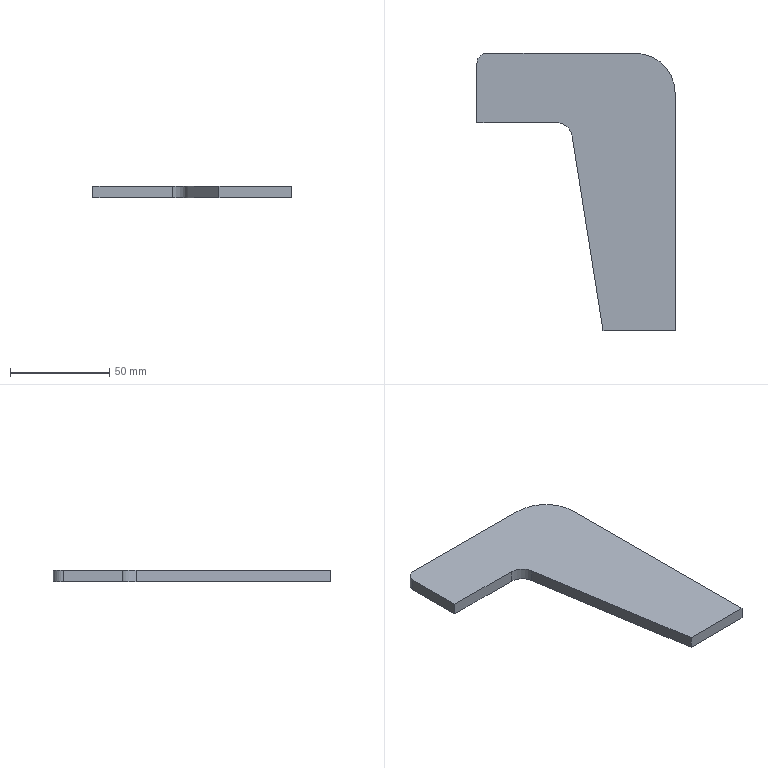Part | STEP file | 02-Reinforcing rib 1 | 1 solid | 11 faces | box 100 x 140 x 6 mm | volume 48661 mm3 | plane 8 | cylinder 3 | commonest cylinder face diameters 10 x1 16 x1 40 x1
STEP:
#1=CARTESIAN_POINT('',(0.,0.,0.));
#2=DIRECTION('',(0.,0.,1.));
#3=DIRECTION('',(1.,0.,0.));
#4=AXIS2_PLACEMENT_3D('',#1,#2,#3);
#5=CARTESIAN_POINT('',(0.,0.,0.));
#6=VERTEX_POINT('',#5);
#7=CARTESIAN_POINT('',(40.167,0.,0.));
#8=VERTEX_POINT('',#7);
#9=CARTESIAN_POINT('',(47.,0.,0.));
#10=DIRECTION('',(1.,0.,0.));
#11=VECTOR('',#10,1.);
#12=LINE('',#9,#11);
#13=CARTESIAN_POINT('',(47.,0.,6.));
#14=DIRECTION('',(0.,1.,0.));
#15=DIRECTION('',(-1.,0.,0.));
#16=AXIS2_PLACEMENT_3D('',#13,#14,#15);
#17=PLANE('',#16);
#18=CARTESIAN_POINT('',(0.,-6.));
#19=DIRECTION('',(-1.,0.));
#20=VECTOR('',#19,1.);
#21=LINE('',#18,#20);
#22=(GEOMETRIC_REPRESENTATION_CONTEXT(2)PARAMETRIC_REPRESENTATION_CONTEXT()REPRESENTATION_CONTEXT('',''));
#23=DEFINITIONAL_REPRESENTATION('',(#21),#22);
#24=PCURVE('',#17,#23);
#25=CARTESIAN_POINT('',(0.,0.,0.));
#26=DIRECTION('',(0.,0.,-1.));
#27=DIRECTION('',(-1.,0.,0.));
#28=AXIS2_PLACEMENT_3D('',#25,#26,#27);
#29=PLANE('',#28);
#30=CARTESIAN_POINT('',(-47.,0.));
#31=DIRECTION('',(-1.,0.));
#32=VECTOR('',#31,1.);
#33=LINE('',#30,#32);
#34=(GEOMETRIC_REPRESENTATION_CONTEXT(2)PARAMETRIC_REPRESENTATION_CONTEXT()REPRESENTATION_CONTEXT('',''));
#35=DEFINITIONAL_REPRESENTATION('',(#33),#34);
#36=PCURVE('',#29,#35);
#37=SURFACE_CURVE('',#12,(#24,#36),.PCURVE_S1.);
#38=EDGE_CURVE('',#6,#8,#37,.T.);
#39=ORIENTED_EDGE('',*,*,#38,.T.);
#40=CARTESIAN_POINT('',(40.167,0.,6.));
#41=VERTEX_POINT('',#40);
#42=CARTESIAN_POINT('',(40.167,0.,6.));
#43=DIRECTION('',(0.,0.,1.));
#44=VECTOR('',#43,1.);
#45=LINE('',#42,#44);
#46=CARTESIAN_POINT('',(6.833,0.));
#47=DIRECTION('',(0.,1.));
#48=VECTOR('',#47,1.);
#49=LINE('',#46,#48);
#50=(GEOMETRIC_REPRESENTATION_CONTEXT(2)PARAMETRIC_REPRESENTATION_CONTEXT()REPRESENTATION_CONTEXT('',''));
#51=DEFINITIONAL_REPRESENTATION('',(#49),#50);
#52=PCURVE('',#17,#51);
#53=CARTESIAN_POINT('',(40.167,-8.,6.));
#54=DIRECTION('',(0.,0.,1.));
#55=DIRECTION('',(1.,0.,0.));
#56=AXIS2_PLACEMENT_3D('',#53,#54,#55);
#57=CYLINDRICAL_SURFACE('',#56,8.);
#58=CARTESIAN_POINT('',(1.571,0.));
#59=DIRECTION('',(0.,1.));
#60=VECTOR('',#59,1.);
#61=LINE('',#58,#60);
#62=(GEOMETRIC_REPRESENTATION_CONTEXT(2)PARAMETRIC_REPRESENTATION_CONTEXT()REPRESENTATION_CONTEXT('',''));
#63=DEFINITIONAL_REPRESENTATION('',(#61),#62);
#64=PCURVE('',#57,#63);
#65=SURFACE_CURVE('',#45,(#52,#64),.PCURVE_S1.);
#66=EDGE_CURVE('',#8,#41,#65,.T.);
#67=ORIENTED_EDGE('',*,*,#66,.T.);
#68=CARTESIAN_POINT('',(0.,0.,6.));
#69=VERTEX_POINT('',#68);
#70=CARTESIAN_POINT('',(47.,0.,6.));
#71=DIRECTION('',(1.,0.,0.));
#72=VECTOR('',#71,1.);
#73=LINE('',#70,#72);
#74=CARTESIAN_POINT('',(0.,0.));
#75=DIRECTION('',(-1.,0.));
#76=VECTOR('',#75,1.);
#77=LINE('',#74,#76);
#78=(GEOMETRIC_REPRESENTATION_CONTEXT(2)PARAMETRIC_REPRESENTATION_CONTEXT()REPRESENTATION_CONTEXT('',''));
#79=DEFINITIONAL_REPRESENTATION('',(#77),#78);
#80=PCURVE('',#17,#79);
#81=CARTESIAN_POINT('',(0.,0.,6.));
#82=DIRECTION('',(0.,0.,-1.));
#83=DIRECTION('',(-1.,0.,0.));
#84=AXIS2_PLACEMENT_3D('',#81,#82,#83);
#85=PLANE('',#84);
#86=CARTESIAN_POINT('',(-47.,0.));
#87=DIRECTION('',(-1.,0.));
#88=VECTOR('',#87,1.);
#89=LINE('',#86,#88);
#90=(GEOMETRIC_REPRESENTATION_CONTEXT(2)PARAMETRIC_REPRESENTATION_CONTEXT()REPRESENTATION_CONTEXT('',''));
#91=DEFINITIONAL_REPRESENTATION('',(#89),#90);
#92=PCURVE('',#85,#91);
#93=SURFACE_CURVE('',#73,(#80,#92),.PCURVE_S1.);
#94=EDGE_CURVE('',#69,#41,#93,.T.);
#95=ORIENTED_EDGE('',*,*,#94,.F.);
#96=CARTESIAN_POINT('',(0.,0.,6.));
#97=DIRECTION('',(0.,0.,-1.));
#98=VECTOR('',#97,1.);
#99=LINE('',#96,#98);
#100=CARTESIAN_POINT('',(47.,0.));
#101=DIRECTION('',(0.,-1.));
#102=VECTOR('',#101,1.);
#103=LINE('',#100,#102);
#104=(GEOMETRIC_REPRESENTATION_CONTEXT(2)PARAMETRIC_REPRESENTATION_CONTEXT()REPRESENTATION_CONTEXT('',''));
#105=DEFINITIONAL_REPRESENTATION('',(#103),#104);
#106=PCURVE('',#17,#105);
#107=CARTESIAN_POINT('',(0.,0.,6.));
#108=DIRECTION('',(1.,0.,0.));
#109=DIRECTION('',(0.,0.,-1.));
#110=AXIS2_PLACEMENT_3D('',#107,#108,#109);
#111=PLANE('',#110);
#112=CARTESIAN_POINT('',(0.,0.));
#113=DIRECTION('',(1.,0.));
#114=VECTOR('',#113,1.);
#115=LINE('',#112,#114);
#116=(GEOMETRIC_REPRESENTATION_CONTEXT(2)PARAMETRIC_REPRESENTATION_CONTEXT()REPRESENTATION_CONTEXT('',''));
#117=DEFINITIONAL_REPRESENTATION('',(#115),#116);
#118=PCURVE('',#111,#117);
#119=SURFACE_CURVE('',#99,(#106,#118),.PCURVE_S1.);
#120=EDGE_CURVE('',#69,#6,#119,.T.);
#121=ORIENTED_EDGE('',*,*,#120,.T.);
#122=EDGE_LOOP('',(#39,#67,#95,#121));
#123=FACE_BOUND('',#122,.T.);
#124=ADVANCED_FACE('',(#123),#17,.F.);
#125=CARTESIAN_POINT('',(48.069,-6.749,6.));
#126=VERTEX_POINT('',#125);
#127=CARTESIAN_POINT('',(63.63,-105.,6.));
#128=VERTEX_POINT('',#127);
#129=CARTESIAN_POINT('',(63.63,-105.,6.));
#130=DIRECTION('',(0.1564,-0.9877,0.));
#131=VECTOR('',#130,1.);
#132=LINE('',#129,#131);
#133=CARTESIAN_POINT('',(63.63,-105.,6.));
#134=DIRECTION('',(0.9877,0.1564,0.));
#135=DIRECTION('',(-0.1564,0.9877,0.));
#136=AXIS2_PLACEMENT_3D('',#133,#134,#135);
#137=PLANE('',#136);
#138=CARTESIAN_POINT('',(0.,0.));
#139=DIRECTION('',(-1.,0.));
#140=VECTOR('',#139,1.);
#141=LINE('',#138,#140);
#142=(GEOMETRIC_REPRESENTATION_CONTEXT(2)PARAMETRIC_REPRESENTATION_CONTEXT()REPRESENTATION_CONTEXT('',''));
#143=DEFINITIONAL_REPRESENTATION('',(#141),#142);
#144=PCURVE('',#137,#143);
#145=CARTESIAN_POINT('',(-63.63,-105.));
#146=DIRECTION('',(-0.1564,-0.9877));
#147=VECTOR('',#146,1.);
#148=LINE('',#145,#147);
#149=(GEOMETRIC_REPRESENTATION_CONTEXT(2)PARAMETRIC_REPRESENTATION_CONTEXT()REPRESENTATION_CONTEXT('',''));
#150=DEFINITIONAL_REPRESENTATION('',(#148),#149);
#151=PCURVE('',#85,#150);
#152=SURFACE_CURVE('',#132,(#144,#151),.PCURVE_S1.);
#153=EDGE_CURVE('',#126,#128,#152,.T.);
#154=ORIENTED_EDGE('',*,*,#153,.F.);
#155=CARTESIAN_POINT('',(48.069,-6.749,0.));
#156=VERTEX_POINT('',#155);
#157=CARTESIAN_POINT('',(48.069,-6.749,0.));
#158=DIRECTION('',(0.,0.,-1.));
#159=VECTOR('',#158,1.);
#160=LINE('',#157,#159);
#161=CARTESIAN_POINT('',(99.476,-6.));
#162=DIRECTION('',(0.,-1.));
#163=VECTOR('',#162,1.);
#164=LINE('',#161,#163);
#165=(GEOMETRIC_REPRESENTATION_CONTEXT(2)PARAMETRIC_REPRESENTATION_CONTEXT()REPRESENTATION_CONTEXT('',''));
#166=DEFINITIONAL_REPRESENTATION('',(#164),#165);
#167=PCURVE('',#137,#166);
#168=CARTESIAN_POINT('',(0.1571,-6.));
#169=DIRECTION('',(0.,-1.));
#170=VECTOR('',#169,1.);
#171=LINE('',#168,#170);
#172=(GEOMETRIC_REPRESENTATION_CONTEXT(2)PARAMETRIC_REPRESENTATION_CONTEXT()REPRESENTATION_CONTEXT('',''));
#173=DEFINITIONAL_REPRESENTATION('',(#171),#172);
#174=PCURVE('',#57,#173);
#175=SURFACE_CURVE('',#160,(#167,#174),.PCURVE_S1.);
#176=EDGE_CURVE('',#126,#156,#175,.T.);
#177=ORIENTED_EDGE('',*,*,#176,.T.);
#178=CARTESIAN_POINT('',(63.63,-105.,0.));
#179=VERTEX_POINT('',#178);
#180=CARTESIAN_POINT('',(63.63,-105.,0.));
#181=DIRECTION('',(0.1564,-0.9877,0.));
#182=VECTOR('',#181,1.);
#183=LINE('',#180,#182);
#184=CARTESIAN_POINT('',(0.,-6.));
#185=DIRECTION('',(-1.,0.));
#186=VECTOR('',#185,1.);
#187=LINE('',#184,#186);
#188=(GEOMETRIC_REPRESENTATION_CONTEXT(2)PARAMETRIC_REPRESENTATION_CONTEXT()REPRESENTATION_CONTEXT('',''));
#189=DEFINITIONAL_REPRESENTATION('',(#187),#188);
#190=PCURVE('',#137,#189);
#191=CARTESIAN_POINT('',(-63.63,-105.));
#192=DIRECTION('',(-0.1564,-0.9877));
#193=VECTOR('',#192,1.);
#194=LINE('',#191,#193);
#195=(GEOMETRIC_REPRESENTATION_CONTEXT(2)PARAMETRIC_REPRESENTATION_CONTEXT()REPRESENTATION_CONTEXT('',''));
#196=DEFINITIONAL_REPRESENTATION('',(#194),#195);
#197=PCURVE('',#29,#196);
#198=SURFACE_CURVE('',#183,(#190,#197),.PCURVE_S1.);
#199=EDGE_CURVE('',#156,#179,#198,.T.);
#200=ORIENTED_EDGE('',*,*,#199,.T.);
#201=CARTESIAN_POINT('',(63.63,-105.,6.));
#202=DIRECTION('',(0.,0.,-1.));
#203=VECTOR('',#202,1.);
#204=LINE('',#201,#203);
#205=CARTESIAN_POINT('',(0.,0.));
#206=DIRECTION('',(0.,-1.));
#207=VECTOR('',#206,1.);
#208=LINE('',#205,#207);
#209=(GEOMETRIC_REPRESENTATION_CONTEXT(2)PARAMETRIC_REPRESENTATION_CONTEXT()REPRESENTATION_CONTEXT('',''));
#210=DEFINITIONAL_REPRESENTATION('',(#208),#209);
#211=PCURVE('',#137,#210);
#212=CARTESIAN_POINT('',(100.,-105.,6.));
#213=DIRECTION('',(0.,1.,0.));
#214=DIRECTION('',(0.,0.,1.));
#215=AXIS2_PLACEMENT_3D('',#212,#213,#214);
#216=PLANE('',#215);
#217=CARTESIAN_POINT('',(0.,-36.37));
#218=DIRECTION('',(-1.,0.));
#219=VECTOR('',#218,1.);
#220=LINE('',#217,#219);
#221=(GEOMETRIC_REPRESENTATION_CONTEXT(2)PARAMETRIC_REPRESENTATION_CONTEXT()REPRESENTATION_CONTEXT('',''));
#222=DEFINITIONAL_REPRESENTATION('',(#220),#221);
#223=PCURVE('',#216,#222);
#224=SURFACE_CURVE('',#204,(#211,#223),.PCURVE_S1.);
#225=EDGE_CURVE('',#128,#179,#224,.T.);
#226=ORIENTED_EDGE('',*,*,#225,.F.);
#227=EDGE_LOOP('',(#154,#177,#200,#226));
#228=FACE_BOUND('',#227,.T.);
#229=ADVANCED_FACE('',(#228),#137,.F.);
#230=CARTESIAN_POINT('',(100.,-105.,0.));
#231=VERTEX_POINT('',#230);
#232=CARTESIAN_POINT('',(100.,-105.,0.));
#233=DIRECTION('',(1.,0.,0.));
#234=VECTOR('',#233,1.);
#235=LINE('',#232,#234);
#236=CARTESIAN_POINT('',(-6.,0.));
#237=DIRECTION('',(0.,1.));
#238=VECTOR('',#237,1.);
#239=LINE('',#236,#238);
#240=(GEOMETRIC_REPRESENTATION_CONTEXT(2)PARAMETRIC_REPRESENTATION_CONTEXT()REPRESENTATION_CONTEXT('',''));
#241=DEFINITIONAL_REPRESENTATION('',(#239),#240);
#242=PCURVE('',#216,#241);
#243=CARTESIAN_POINT('',(-100.,-105.));
#244=DIRECTION('',(-1.,0.));
#245=VECTOR('',#244,1.);
#246=LINE('',#243,#245);
#247=(GEOMETRIC_REPRESENTATION_CONTEXT(2)PARAMETRIC_REPRESENTATION_CONTEXT()REPRESENTATION_CONTEXT('',''));
#248=DEFINITIONAL_REPRESENTATION('',(#246),#247);
#249=PCURVE('',#29,#248);
#250=SURFACE_CURVE('',#235,(#242,#249),.PCURVE_S1.);
#251=EDGE_CURVE('',#179,#231,#250,.T.);
#252=ORIENTED_EDGE('',*,*,#251,.T.);
#253=CARTESIAN_POINT('',(100.,-105.,6.));
#254=VERTEX_POINT('',#253);
#255=CARTESIAN_POINT('',(100.,-105.,6.));
#256=DIRECTION('',(0.,0.,-1.));
#257=VECTOR('',#256,1.);
#258=LINE('',#255,#257);
#259=CARTESIAN_POINT('',(0.,0.));
#260=DIRECTION('',(-1.,0.));
#261=VECTOR('',#260,1.);
#262=LINE('',#259,#261);
#263=(GEOMETRIC_REPRESENTATION_CONTEXT(2)PARAMETRIC_REPRESENTATION_CONTEXT()REPRESENTATION_CONTEXT('',''));
#264=DEFINITIONAL_REPRESENTATION('',(#262),#263);
#265=PCURVE('',#216,#264);
#266=CARTESIAN_POINT('',(100.,35.,6.));
#267=DIRECTION('',(-1.,0.,0.));
#268=DIRECTION('',(0.,-1.,0.));
#269=AXIS2_PLACEMENT_3D('',#266,#267,#268);
#270=PLANE('',#269);
#271=CARTESIAN_POINT('',(140.,0.));
#272=DIRECTION('',(0.,-1.));
#273=VECTOR('',#272,1.);
#274=LINE('',#271,#273);
#275=(GEOMETRIC_REPRESENTATION_CONTEXT(2)PARAMETRIC_REPRESENTATION_CONTEXT()REPRESENTATION_CONTEXT('',''));
#276=DEFINITIONAL_REPRESENTATION('',(#274),#275);
#277=PCURVE('',#270,#276);
#278=SURFACE_CURVE('',#258,(#265,#277),.PCURVE_S1.);
#279=EDGE_CURVE('',#254,#231,#278,.T.);
#280=ORIENTED_EDGE('',*,*,#279,.F.);
#281=CARTESIAN_POINT('',(100.,-105.,6.));
#282=DIRECTION('',(1.,0.,0.));
#283=VECTOR('',#282,1.);
#284=LINE('',#281,#283);
#285=CARTESIAN_POINT('',(0.,0.));
#286=DIRECTION('',(0.,1.));
#287=VECTOR('',#286,1.);
#288=LINE('',#285,#287);
#289=(GEOMETRIC_REPRESENTATION_CONTEXT(2)PARAMETRIC_REPRESENTATION_CONTEXT()REPRESENTATION_CONTEXT('',''));
#290=DEFINITIONAL_REPRESENTATION('',(#288),#289);
#291=PCURVE('',#216,#290);
#292=CARTESIAN_POINT('',(-100.,-105.));
#293=DIRECTION('',(-1.,0.));
#294=VECTOR('',#293,1.);
#295=LINE('',#292,#294);
#296=(GEOMETRIC_REPRESENTATION_CONTEXT(2)PARAMETRIC_REPRESENTATION_CONTEXT()REPRESENTATION_CONTEXT('',''));
#297=DEFINITIONAL_REPRESENTATION('',(#295),#296);
#298=PCURVE('',#85,#297);
#299=SURFACE_CURVE('',#284,(#291,#298),.PCURVE_S1.);
#300=EDGE_CURVE('',#128,#254,#299,.T.);
#301=ORIENTED_EDGE('',*,*,#300,.F.);
#302=ORIENTED_EDGE('',*,*,#225,.T.);
#303=EDGE_LOOP('',(#252,#280,#301,#302));
#304=FACE_BOUND('',#303,.T.);
#305=ADVANCED_FACE('',(#304),#216,.F.);
#306=CARTESIAN_POINT('',(100.,15.,0.));
#307=VERTEX_POINT('',#306);
#308=CARTESIAN_POINT('',(100.,35.,0.));
#309=DIRECTION('',(0.,1.,0.));
#310=VECTOR('',#309,1.);
#311=LINE('',#308,#310);
#312=CARTESIAN_POINT('',(0.,-6.));
#313=DIRECTION('',(-1.,0.));
#314=VECTOR('',#313,1.);
#315=LINE('',#312,#314);
#316=(GEOMETRIC_REPRESENTATION_CONTEXT(2)PARAMETRIC_REPRESENTATION_CONTEXT()REPRESENTATION_CONTEXT('',''));
#317=DEFINITIONAL_REPRESENTATION('',(#315),#316);
#318=PCURVE('',#270,#317);
#319=CARTESIAN_POINT('',(-100.,35.));
#320=DIRECTION('',(0.,1.));
#321=VECTOR('',#320,1.);
#322=LINE('',#319,#321);
#323=(GEOMETRIC_REPRESENTATION_CONTEXT(2)PARAMETRIC_REPRESENTATION_CONTEXT()REPRESENTATION_CONTEXT('',''));
#324=DEFINITIONAL_REPRESENTATION('',(#322),#323);
#325=PCURVE('',#29,#324);
#326=SURFACE_CURVE('',#311,(#318,#325),.PCURVE_S1.);
#327=EDGE_CURVE('',#231,#307,#326,.T.);
#328=ORIENTED_EDGE('',*,*,#327,.T.);
#329=CARTESIAN_POINT('',(100.,15.,6.));
#330=VERTEX_POINT('',#329);
#331=CARTESIAN_POINT('',(100.,15.,6.));
#332=DIRECTION('',(0.,0.,1.));
#333=VECTOR('',#332,1.);
#334=LINE('',#331,#333);
#335=CARTESIAN_POINT('',(20.,0.));
#336=DIRECTION('',(0.,1.));
#337=VECTOR('',#336,1.);
#338=LINE('',#335,#337);
#339=(GEOMETRIC_REPRESENTATION_CONTEXT(2)PARAMETRIC_REPRESENTATION_CONTEXT()REPRESENTATION_CONTEXT('',''));
#340=DEFINITIONAL_REPRESENTATION('',(#338),#339);
#341=PCURVE('',#270,#340);
#342=CARTESIAN_POINT('',(80.,15.,6.));
#343=DIRECTION('',(0.,0.,-1.));
#344=DIRECTION('',(-1.,0.,0.));
#345=AXIS2_PLACEMENT_3D('',#342,#343,#344);
#346=CYLINDRICAL_SURFACE('',#345,20.);
#347=CARTESIAN_POINT('',(3.142,0.));
#348=DIRECTION('',(0.,-1.));
#349=VECTOR('',#348,1.);
#350=LINE('',#347,#349);
#351=(GEOMETRIC_REPRESENTATION_CONTEXT(2)PARAMETRIC_REPRESENTATION_CONTEXT()REPRESENTATION_CONTEXT('',''));
#352=DEFINITIONAL_REPRESENTATION('',(#350),#351);
#353=PCURVE('',#346,#352);
#354=SURFACE_CURVE('',#334,(#341,#353),.PCURVE_S1.);
#355=EDGE_CURVE('',#307,#330,#354,.T.);
#356=ORIENTED_EDGE('',*,*,#355,.T.);
#357=CARTESIAN_POINT('',(100.,35.,6.));
#358=DIRECTION('',(0.,1.,0.));
#359=VECTOR('',#358,1.);
#360=LINE('',#357,#359);
#361=CARTESIAN_POINT('',(0.,0.));
#362=DIRECTION('',(-1.,0.));
#363=VECTOR('',#362,1.);
#364=LINE('',#361,#363);
#365=(GEOMETRIC_REPRESENTATION_CONTEXT(2)PARAMETRIC_REPRESENTATION_CONTEXT()REPRESENTATION_CONTEXT('',''));
#366=DEFINITIONAL_REPRESENTATION('',(#364),#365);
#367=PCURVE('',#270,#366);
#368=CARTESIAN_POINT('',(-100.,35.));
#369=DIRECTION('',(0.,1.));
#370=VECTOR('',#369,1.);
#371=LINE('',#368,#370);
#372=(GEOMETRIC_REPRESENTATION_CONTEXT(2)PARAMETRIC_REPRESENTATION_CONTEXT()REPRESENTATION_CONTEXT('',''));
#373=DEFINITIONAL_REPRESENTATION('',(#371),#372);
#374=PCURVE('',#85,#373);
#375=SURFACE_CURVE('',#360,(#367,#374),.PCURVE_S1.);
#376=EDGE_CURVE('',#254,#330,#375,.T.);
#377=ORIENTED_EDGE('',*,*,#376,.F.);
#378=ORIENTED_EDGE('',*,*,#279,.T.);
#379=EDGE_LOOP('',(#328,#356,#377,#378));
#380=FACE_BOUND('',#379,.T.);
#381=ADVANCED_FACE('',(#380),#270,.F.);
#382=CARTESIAN_POINT('',(80.,35.,0.));
#383=VERTEX_POINT('',#382);
#384=CARTESIAN_POINT('',(5.,35.,0.));
#385=VERTEX_POINT('',#384);
#386=CARTESIAN_POINT('',(0.,35.,0.));
#387=DIRECTION('',(-1.,0.,0.));
#388=VECTOR('',#387,1.);
#389=LINE('',#386,#388);
#390=CARTESIAN_POINT('',(0.,35.,6.));
#391=DIRECTION('',(0.,-1.,0.));
#392=DIRECTION('',(0.,0.,-1.));
#393=AXIS2_PLACEMENT_3D('',#390,#391,#392);
#394=PLANE('',#393);
#395=CARTESIAN_POINT('',(6.,0.));
#396=DIRECTION('',(0.,-1.));
#397=VECTOR('',#396,1.);
#398=LINE('',#395,#397);
#399=(GEOMETRIC_REPRESENTATION_CONTEXT(2)PARAMETRIC_REPRESENTATION_CONTEXT()REPRESENTATION_CONTEXT('',''));
#400=DEFINITIONAL_REPRESENTATION('',(#398),#399);
#401=PCURVE('',#394,#400);
#402=CARTESIAN_POINT('',(0.,35.));
#403=DIRECTION('',(1.,0.));
#404=VECTOR('',#403,1.);
#405=LINE('',#402,#404);
#406=(GEOMETRIC_REPRESENTATION_CONTEXT(2)PARAMETRIC_REPRESENTATION_CONTEXT()REPRESENTATION_CONTEXT('',''));
#407=DEFINITIONAL_REPRESENTATION('',(#405),#406);
#408=PCURVE('',#29,#407);
#409=SURFACE_CURVE('',#389,(#401,#408),.PCURVE_S1.);
#410=EDGE_CURVE('',#383,#385,#409,.T.);
#411=ORIENTED_EDGE('',*,*,#410,.T.);
#412=CARTESIAN_POINT('',(5.,35.,6.));
#413=VERTEX_POINT('',#412);
#414=CARTESIAN_POINT('',(5.,35.,6.));
#415=DIRECTION('',(0.,0.,1.));
#416=VECTOR('',#415,1.);
#417=LINE('',#414,#416);
#418=CARTESIAN_POINT('',(0.,5.));
#419=DIRECTION('',(-1.,0.));
#420=VECTOR('',#419,1.);
#421=LINE('',#418,#420);
#422=(GEOMETRIC_REPRESENTATION_CONTEXT(2)PARAMETRIC_REPRESENTATION_CONTEXT()REPRESENTATION_CONTEXT('',''));
#423=DEFINITIONAL_REPRESENTATION('',(#421),#422);
#424=PCURVE('',#394,#423);
#425=CARTESIAN_POINT('',(5.,30.,6.));
#426=DIRECTION('',(0.,0.,-1.));
#427=DIRECTION('',(-1.,0.,0.));
#428=AXIS2_PLACEMENT_3D('',#425,#426,#427);
#429=CYLINDRICAL_SURFACE('',#428,5.);
#430=CARTESIAN_POINT('',(1.571,0.));
#431=DIRECTION('',(0.,-1.));
#432=VECTOR('',#431,1.);
#433=LINE('',#430,#432);
#434=(GEOMETRIC_REPRESENTATION_CONTEXT(2)PARAMETRIC_REPRESENTATION_CONTEXT()REPRESENTATION_CONTEXT('',''));
#435=DEFINITIONAL_REPRESENTATION('',(#433),#434);
#436=PCURVE('',#429,#435);
#437=SURFACE_CURVE('',#417,(#424,#436),.PCURVE_S1.);
#438=EDGE_CURVE('',#385,#413,#437,.T.);
#439=ORIENTED_EDGE('',*,*,#438,.T.);
#440=CARTESIAN_POINT('',(80.,35.,6.));
#441=VERTEX_POINT('',#440);
#442=CARTESIAN_POINT('',(0.,35.,6.));
#443=DIRECTION('',(-1.,0.,0.));
#444=VECTOR('',#443,1.);
#445=LINE('',#442,#444);
#446=CARTESIAN_POINT('',(0.,0.));
#447=DIRECTION('',(0.,-1.));
#448=VECTOR('',#447,1.);
#449=LINE('',#446,#448);
#450=(GEOMETRIC_REPRESENTATION_CONTEXT(2)PARAMETRIC_REPRESENTATION_CONTEXT()REPRESENTATION_CONTEXT('',''));
#451=DEFINITIONAL_REPRESENTATION('',(#449),#450);
#452=PCURVE('',#394,#451);
#453=CARTESIAN_POINT('',(0.,35.));
#454=DIRECTION('',(1.,0.));
#455=VECTOR('',#454,1.);
#456=LINE('',#453,#455);
#457=(GEOMETRIC_REPRESENTATION_CONTEXT(2)PARAMETRIC_REPRESENTATION_CONTEXT()REPRESENTATION_CONTEXT('',''));
#458=DEFINITIONAL_REPRESENTATION('',(#456),#457);
#459=PCURVE('',#85,#458);
#460=SURFACE_CURVE('',#445,(#452,#459),.PCURVE_S1.);
#461=EDGE_CURVE('',#441,#413,#460,.T.);
#462=ORIENTED_EDGE('',*,*,#461,.F.);
#463=CARTESIAN_POINT('',(80.,35.,6.));
#464=DIRECTION('',(0.,0.,-1.));
#465=VECTOR('',#464,1.);
#466=LINE('',#463,#465);
#467=CARTESIAN_POINT('',(0.,80.));
#468=DIRECTION('',(1.,0.));
#469=VECTOR('',#468,1.);
#470=LINE('',#467,#469);
#471=(GEOMETRIC_REPRESENTATION_CONTEXT(2)PARAMETRIC_REPRESENTATION_CONTEXT()REPRESENTATION_CONTEXT('',''));
#472=DEFINITIONAL_REPRESENTATION('',(#470),#471);
#473=PCURVE('',#394,#472);
#474=CARTESIAN_POINT('',(1.571,0.));
#475=DIRECTION('',(0.,1.));
#476=VECTOR('',#475,1.);
#477=LINE('',#474,#476);
#478=(GEOMETRIC_REPRESENTATION_CONTEXT(2)PARAMETRIC_REPRESENTATION_CONTEXT()REPRESENTATION_CONTEXT('',''));
#479=DEFINITIONAL_REPRESENTATION('',(#477),#478);
#480=PCURVE('',#346,#479);
#481=SURFACE_CURVE('',#466,(#473,#480),.PCURVE_S1.);
#482=EDGE_CURVE('',#441,#383,#481,.T.);
#483=ORIENTED_EDGE('',*,*,#482,.T.);
#484=EDGE_LOOP('',(#411,#439,#462,#483));
#485=FACE_BOUND('',#484,.T.);
#486=ADVANCED_FACE('',(#485),#394,.F.);
#487=CARTESIAN_POINT('',(0.,30.,6.));
#488=VERTEX_POINT('',#487);
#489=CARTESIAN_POINT('',(0.,0.,6.));
#490=DIRECTION('',(0.,-1.,0.));
#491=VECTOR('',#490,1.);
#492=LINE('',#489,#491);
#493=CARTESIAN_POINT('',(0.,0.));
#494=DIRECTION('',(0.,-1.));
#495=VECTOR('',#494,1.);
#496=LINE('',#493,#495);
#497=(GEOMETRIC_REPRESENTATION_CONTEXT(2)PARAMETRIC_REPRESENTATION_CONTEXT()REPRESENTATION_CONTEXT('',''));
#498=DEFINITIONAL_REPRESENTATION('',(#496),#497);
#499=PCURVE('',#111,#498);
#500=CARTESIAN_POINT('',(0.,0.));
#501=DIRECTION('',(0.,-1.));
#502=VECTOR('',#501,1.);
#503=LINE('',#500,#502);
#504=(GEOMETRIC_REPRESENTATION_CONTEXT(2)PARAMETRIC_REPRESENTATION_CONTEXT()REPRESENTATION_CONTEXT('',''));
#505=DEFINITIONAL_REPRESENTATION('',(#503),#504);
#506=PCURVE('',#85,#505);
#507=SURFACE_CURVE('',#492,(#499,#506),.PCURVE_S1.);
#508=EDGE_CURVE('',#488,#69,#507,.T.);
#509=ORIENTED_EDGE('',*,*,#508,.F.);
#510=CARTESIAN_POINT('',(0.,30.,0.));
#511=VERTEX_POINT('',#510);
#512=CARTESIAN_POINT('',(0.,30.,6.));
#513=DIRECTION('',(0.,0.,-1.));
#514=VECTOR('',#513,1.);
#515=LINE('',#512,#514);
#516=CARTESIAN_POINT('',(0.,30.));
#517=DIRECTION('',(1.,0.));
#518=VECTOR('',#517,1.);
#519=LINE('',#516,#518);
#520=(GEOMETRIC_REPRESENTATION_CONTEXT(2)PARAMETRIC_REPRESENTATION_CONTEXT()REPRESENTATION_CONTEXT('',''));
#521=DEFINITIONAL_REPRESENTATION('',(#519),#520);
#522=PCURVE('',#111,#521);
#523=CARTESIAN_POINT('',(0.,0.));
#524=DIRECTION('',(0.,1.));
#525=VECTOR('',#524,1.);
#526=LINE('',#523,#525);
#527=(GEOMETRIC_REPRESENTATION_CONTEXT(2)PARAMETRIC_REPRESENTATION_CONTEXT()REPRESENTATION_CONTEXT('',''));
#528=DEFINITIONAL_REPRESENTATION('',(#526),#527);
#529=PCURVE('',#429,#528);
#530=SURFACE_CURVE('',#515,(#522,#529),.PCURVE_S1.);
#531=EDGE_CURVE('',#488,#511,#530,.T.);
#532=ORIENTED_EDGE('',*,*,#531,.T.);
#533=CARTESIAN_POINT('',(0.,0.,0.));
#534=DIRECTION('',(0.,-1.,0.));
#535=VECTOR('',#534,1.);
#536=LINE('',#533,#535);
#537=CARTESIAN_POINT('',(6.,0.));
#538=DIRECTION('',(0.,-1.));
#539=VECTOR('',#538,1.);
#540=LINE('',#537,#539);
#541=(GEOMETRIC_REPRESENTATION_CONTEXT(2)PARAMETRIC_REPRESENTATION_CONTEXT()REPRESENTATION_CONTEXT('',''));
#542=DEFINITIONAL_REPRESENTATION('',(#540),#541);
#543=PCURVE('',#111,#542);
#544=CARTESIAN_POINT('',(0.,0.));
#545=DIRECTION('',(0.,-1.));
#546=VECTOR('',#545,1.);
#547=LINE('',#544,#546);
#548=(GEOMETRIC_REPRESENTATION_CONTEXT(2)PARAMETRIC_REPRESENTATION_CONTEXT()REPRESENTATION_CONTEXT('',''));
#549=DEFINITIONAL_REPRESENTATION('',(#547),#548);
#550=PCURVE('',#29,#549);
#551=SURFACE_CURVE('',#536,(#543,#550),.PCURVE_S1.);
#552=EDGE_CURVE('',#511,#6,#551,.T.);
#553=ORIENTED_EDGE('',*,*,#552,.T.);
#554=ORIENTED_EDGE('',*,*,#120,.F.);
#555=EDGE_LOOP('',(#509,#532,#553,#554));
#556=FACE_BOUND('',#555,.T.);
#557=ADVANCED_FACE('',(#556),#111,.F.);
#558=ORIENTED_EDGE('',*,*,#461,.T.);
#559=CARTESIAN_POINT('',(5.,30.,6.));
#560=DIRECTION('',(0.,0.,1.));
#561=DIRECTION('',(-1.,0.,0.));
#562=AXIS2_PLACEMENT_3D('',#559,#560,#561);
#563=CIRCLE('',#562,5.);
#564=CARTESIAN_POINT('',(0.,30.));
#565=CARTESIAN_POINT('',(0.,21.34));
#566=CARTESIAN_POINT('',(-7.5,25.67));
#567=CARTESIAN_POINT('',(-15.,30.));
#568=CARTESIAN_POINT('',(-7.5,34.33));
#569=CARTESIAN_POINT('',(0.,38.66));
#570=CARTESIAN_POINT('',(0.,30.));
#571=(BOUNDED_CURVE()B_SPLINE_CURVE(2,(#564,#565,#566,#567,#568,#569,#570),.UNSPECIFIED.,.T.,.F.)B_SPLINE_CURVE_WITH_KNOTS((1,2,2,2,2,1),(-2.094,0.,2.094,4.189,6.283,8.378),.UNSPECIFIED.)CURVE()GEOMETRIC_REPRESENTATION_ITEM()RATIONAL_B_SPLINE_CURVE((1.,0.5,1.,0.5,1.,0.5,1.))REPRESENTATION_ITEM(''));
#572=(GEOMETRIC_REPRESENTATION_CONTEXT(2)PARAMETRIC_REPRESENTATION_CONTEXT()REPRESENTATION_CONTEXT('',''));
#573=DEFINITIONAL_REPRESENTATION('',(#571),#572);
#574=PCURVE('',#85,#573);
#575=CARTESIAN_POINT('',(6.283,0.));
#576=DIRECTION('',(-1.,0.));
#577=VECTOR('',#576,1.);
#578=LINE('',#575,#577);
#579=(GEOMETRIC_REPRESENTATION_CONTEXT(2)PARAMETRIC_REPRESENTATION_CONTEXT()REPRESENTATION_CONTEXT('',''));
#580=DEFINITIONAL_REPRESENTATION('',(#578),#579);
#581=PCURVE('',#429,#580);
#582=SURFACE_CURVE('',#563,(#574,#581),.PCURVE_S1.);
#583=EDGE_CURVE('',#413,#488,#582,.T.);
#584=ORIENTED_EDGE('',*,*,#583,.T.);
#585=ORIENTED_EDGE('',*,*,#508,.T.);
#586=ORIENTED_EDGE('',*,*,#94,.T.);
#587=CARTESIAN_POINT('',(40.167,-8.,6.));
#588=DIRECTION('',(0.,0.,-1.));
#589=DIRECTION('',(-1.,0.,0.));
#590=AXIS2_PLACEMENT_3D('',#587,#588,#589);
#591=CIRCLE('',#590,8.);
#592=CARTESIAN_POINT('',(-40.167,-8.));
#593=DIRECTION('',(1.,0.));
#594=AXIS2_PLACEMENT_2D('',#592,#593);
#595=CIRCLE('',#594,8.);
#596=(GEOMETRIC_REPRESENTATION_CONTEXT(2)PARAMETRIC_REPRESENTATION_CONTEXT()REPRESENTATION_CONTEXT('',''));
#597=DEFINITIONAL_REPRESENTATION('',(#595),#596);
#598=PCURVE('',#85,#597);
#599=CARTESIAN_POINT('',(3.142,0.));
#600=DIRECTION('',(-1.,0.));
#601=VECTOR('',#600,1.);
#602=LINE('',#599,#601);
#603=(GEOMETRIC_REPRESENTATION_CONTEXT(2)PARAMETRIC_REPRESENTATION_CONTEXT()REPRESENTATION_CONTEXT('',''));
#604=DEFINITIONAL_REPRESENTATION('',(#602),#603);
#605=PCURVE('',#57,#604);
#606=SURFACE_CURVE('',#591,(#598,#605),.PCURVE_S1.);
#607=EDGE_CURVE('',#41,#126,#606,.T.);
#608=ORIENTED_EDGE('',*,*,#607,.T.);
#609=ORIENTED_EDGE('',*,*,#153,.T.);
#610=ORIENTED_EDGE('',*,*,#300,.T.);
#611=ORIENTED_EDGE('',*,*,#376,.T.);
#612=CARTESIAN_POINT('',(80.,15.,6.));
#613=DIRECTION('',(0.,0.,1.));
#614=DIRECTION('',(-1.,0.,0.));
#615=AXIS2_PLACEMENT_3D('',#612,#613,#614);
#616=CIRCLE('',#615,20.);
#617=CARTESIAN_POINT('',(-60.,15.));
#618=CARTESIAN_POINT('',(-60.,-19.641));
#619=CARTESIAN_POINT('',(-90.,-2.321));
#620=CARTESIAN_POINT('',(-120.,15.));
#621=CARTESIAN_POINT('',(-90.,32.321));
#622=CARTESIAN_POINT('',(-60.,49.641));
#623=CARTESIAN_POINT('',(-60.,15.));
#624=(BOUNDED_CURVE()B_SPLINE_CURVE(2,(#617,#618,#619,#620,#621,#622,#623),.UNSPECIFIED.,.T.,.F.)B_SPLINE_CURVE_WITH_KNOTS((1,2,2,2,2,1),(-2.094,0.,2.094,4.189,6.283,8.378),.UNSPECIFIED.)CURVE()GEOMETRIC_REPRESENTATION_ITEM()RATIONAL_B_SPLINE_CURVE((1.,0.5,1.,0.5,1.,0.5,1.))REPRESENTATION_ITEM(''));
#625=(GEOMETRIC_REPRESENTATION_CONTEXT(2)PARAMETRIC_REPRESENTATION_CONTEXT()REPRESENTATION_CONTEXT('',''));
#626=DEFINITIONAL_REPRESENTATION('',(#624),#625);
#627=PCURVE('',#85,#626);
#628=CARTESIAN_POINT('',(6.283,0.));
#629=DIRECTION('',(-1.,0.));
#630=VECTOR('',#629,1.);
#631=LINE('',#628,#630);
#632=(GEOMETRIC_REPRESENTATION_CONTEXT(2)PARAMETRIC_REPRESENTATION_CONTEXT()REPRESENTATION_CONTEXT('',''));
#633=DEFINITIONAL_REPRESENTATION('',(#631),#632);
#634=PCURVE('',#346,#633);
#635=SURFACE_CURVE('',#616,(#627,#634),.PCURVE_S1.);
#636=EDGE_CURVE('',#330,#441,#635,.T.);
#637=ORIENTED_EDGE('',*,*,#636,.T.);
#638=EDGE_LOOP('',(#558,#584,#585,#586,#608,#609,#610,#611,#637));
#639=FACE_BOUND('',#638,.T.);
#640=ADVANCED_FACE('',(#639),#85,.F.);
#641=ORIENTED_EDGE('',*,*,#552,.F.);
#642=CARTESIAN_POINT('',(5.,30.,0.));
#643=DIRECTION('',(0.,0.,-1.));
#644=DIRECTION('',(-1.,0.,0.));
#645=AXIS2_PLACEMENT_3D('',#642,#643,#644);
#646=CIRCLE('',#645,5.);
#647=CARTESIAN_POINT('',(-5.,30.));
#648=DIRECTION('',(1.,0.));
#649=AXIS2_PLACEMENT_2D('',#647,#648);
#650=CIRCLE('',#649,5.);
#651=(GEOMETRIC_REPRESENTATION_CONTEXT(2)PARAMETRIC_REPRESENTATION_CONTEXT()REPRESENTATION_CONTEXT('',''));
#652=DEFINITIONAL_REPRESENTATION('',(#650),#651);
#653=PCURVE('',#29,#652);
#654=CARTESIAN_POINT('',(0.,6.));
#655=DIRECTION('',(1.,0.));
#656=VECTOR('',#655,1.);
#657=LINE('',#654,#656);
#658=(GEOMETRIC_REPRESENTATION_CONTEXT(2)PARAMETRIC_REPRESENTATION_CONTEXT()REPRESENTATION_CONTEXT('',''));
#659=DEFINITIONAL_REPRESENTATION('',(#657),#658);
#660=PCURVE('',#429,#659);
#661=SURFACE_CURVE('',#646,(#653,#660),.PCURVE_S1.);
#662=EDGE_CURVE('',#511,#385,#661,.T.);
#663=ORIENTED_EDGE('',*,*,#662,.T.);
#664=ORIENTED_EDGE('',*,*,#410,.F.);
#665=CARTESIAN_POINT('',(80.,15.,0.));
#666=DIRECTION('',(0.,0.,-1.));
#667=DIRECTION('',(-1.,0.,0.));
#668=AXIS2_PLACEMENT_3D('',#665,#666,#667);
#669=CIRCLE('',#668,20.);
#670=CARTESIAN_POINT('',(-80.,15.));
#671=DIRECTION('',(1.,0.));
#672=AXIS2_PLACEMENT_2D('',#670,#671);
#673=CIRCLE('',#672,20.);
#674=(GEOMETRIC_REPRESENTATION_CONTEXT(2)PARAMETRIC_REPRESENTATION_CONTEXT()REPRESENTATION_CONTEXT('',''));
#675=DEFINITIONAL_REPRESENTATION('',(#673),#674);
#676=PCURVE('',#29,#675);
#677=CARTESIAN_POINT('',(0.,6.));
#678=DIRECTION('',(1.,0.));
#679=VECTOR('',#678,1.);
#680=LINE('',#677,#679);
#681=(GEOMETRIC_REPRESENTATION_CONTEXT(2)PARAMETRIC_REPRESENTATION_CONTEXT()REPRESENTATION_CONTEXT('',''));
#682=DEFINITIONAL_REPRESENTATION('',(#680),#681);
#683=PCURVE('',#346,#682);
#684=SURFACE_CURVE('',#669,(#676,#683),.PCURVE_S1.);
#685=EDGE_CURVE('',#383,#307,#684,.T.);
#686=ORIENTED_EDGE('',*,*,#685,.T.);
#687=ORIENTED_EDGE('',*,*,#327,.F.);
#688=ORIENTED_EDGE('',*,*,#251,.F.);
#689=ORIENTED_EDGE('',*,*,#199,.F.);
#690=CARTESIAN_POINT('',(40.167,-8.,0.));
#691=DIRECTION('',(0.,0.,1.));
#692=DIRECTION('',(-1.,0.,0.));
#693=AXIS2_PLACEMENT_3D('',#690,#691,#692);
#694=CIRCLE('',#693,8.);
#695=CARTESIAN_POINT('',(-32.167,-8.));
#696=CARTESIAN_POINT('',(-32.167,-21.856));
#697=CARTESIAN_POINT('',(-44.167,-14.928));
#698=CARTESIAN_POINT('',(-56.167,-8.));
#699=CARTESIAN_POINT('',(-44.167,-1.072));
#700=CARTESIAN_POINT('',(-32.167,5.856));
#701=CARTESIAN_POINT('',(-32.167,-8.));
#702=(BOUNDED_CURVE()B_SPLINE_CURVE(2,(#695,#696,#697,#698,#699,#700,#701),.UNSPECIFIED.,.T.,.F.)B_SPLINE_CURVE_WITH_KNOTS((1,2,2,2,2,1),(-2.094,0.,2.094,4.189,6.283,8.378),.UNSPECIFIED.)CURVE()GEOMETRIC_REPRESENTATION_ITEM()RATIONAL_B_SPLINE_CURVE((1.,0.5,1.,0.5,1.,0.5,1.))REPRESENTATION_ITEM(''));
#703=(GEOMETRIC_REPRESENTATION_CONTEXT(2)PARAMETRIC_REPRESENTATION_CONTEXT()REPRESENTATION_CONTEXT('',''));
#704=DEFINITIONAL_REPRESENTATION('',(#702),#703);
#705=PCURVE('',#29,#704);
#706=CARTESIAN_POINT('',(-3.142,-6.));
#707=DIRECTION('',(1.,0.));
#708=VECTOR('',#707,1.);
#709=LINE('',#706,#708);
#710=(GEOMETRIC_REPRESENTATION_CONTEXT(2)PARAMETRIC_REPRESENTATION_CONTEXT()REPRESENTATION_CONTEXT('',''));
#711=DEFINITIONAL_REPRESENTATION('',(#709),#710);
#712=PCURVE('',#57,#711);
#713=SURFACE_CURVE('',#694,(#705,#712),.PCURVE_S1.);
#714=EDGE_CURVE('',#156,#8,#713,.T.);
#715=ORIENTED_EDGE('',*,*,#714,.T.);
#716=ORIENTED_EDGE('',*,*,#38,.F.);
#717=EDGE_LOOP('',(#641,#663,#664,#686,#687,#688,#689,#715,#716));
#718=FACE_BOUND('',#717,.T.);
#719=ADVANCED_FACE('',(#718),#29,.T.);
#720=ORIENTED_EDGE('',*,*,#636,.F.);
#721=ORIENTED_EDGE('',*,*,#355,.F.);
#722=ORIENTED_EDGE('',*,*,#685,.F.);
#723=ORIENTED_EDGE('',*,*,#482,.F.);
#724=EDGE_LOOP('',(#720,#721,#722,#723));
#725=FACE_BOUND('',#724,.T.);
#726=ADVANCED_FACE('',(#725),#346,.T.);
#727=ORIENTED_EDGE('',*,*,#583,.F.);
#728=ORIENTED_EDGE('',*,*,#438,.F.);
#729=ORIENTED_EDGE('',*,*,#662,.F.);
#730=ORIENTED_EDGE('',*,*,#531,.F.);
#731=EDGE_LOOP('',(#727,#728,#729,#730));
#732=FACE_BOUND('',#731,.T.);
#733=ADVANCED_FACE('',(#732),#429,.T.);
#734=ORIENTED_EDGE('',*,*,#176,.T.);
#735=ORIENTED_EDGE('',*,*,#714,.T.);
#736=ORIENTED_EDGE('',*,*,#66,.T.);
#737=ORIENTED_EDGE('',*,*,#607,.T.);
#738=EDGE_LOOP('',(#734,#735,#736,#737));
#739=FACE_BOUND('',#738,.F.);
#740=ADVANCED_FACE('',(#739),#57,.F.);
#741=CLOSED_SHELL('',(#124,#229,#305,#381,#486,#557,#640,#719,#726,#733,#740));
#742=MANIFOLD_SOLID_BREP('',#741);
#743=(LENGTH_UNIT()NAMED_UNIT(*)SI_UNIT(.MILLI.,.METRE.));
#744=UNCERTAINTY_MEASURE_WITH_UNIT(LENGTH_MEASURE(0.0000001),#743,'','');
#745=(NAMED_UNIT(*)PLANE_ANGLE_UNIT()SI_UNIT($,.RADIAN.));
#746=(NAMED_UNIT(*)SI_UNIT($,.STERADIAN.)SOLID_ANGLE_UNIT());
#747=(GEOMETRIC_REPRESENTATION_CONTEXT(3)GLOBAL_UNCERTAINTY_ASSIGNED_CONTEXT((#744))GLOBAL_UNIT_ASSIGNED_CONTEXT((#743,#745,#746))REPRESENTATION_CONTEXT('',''));
#748=ADVANCED_BREP_SHAPE_REPRESENTATION('',(#4,#742),#747);